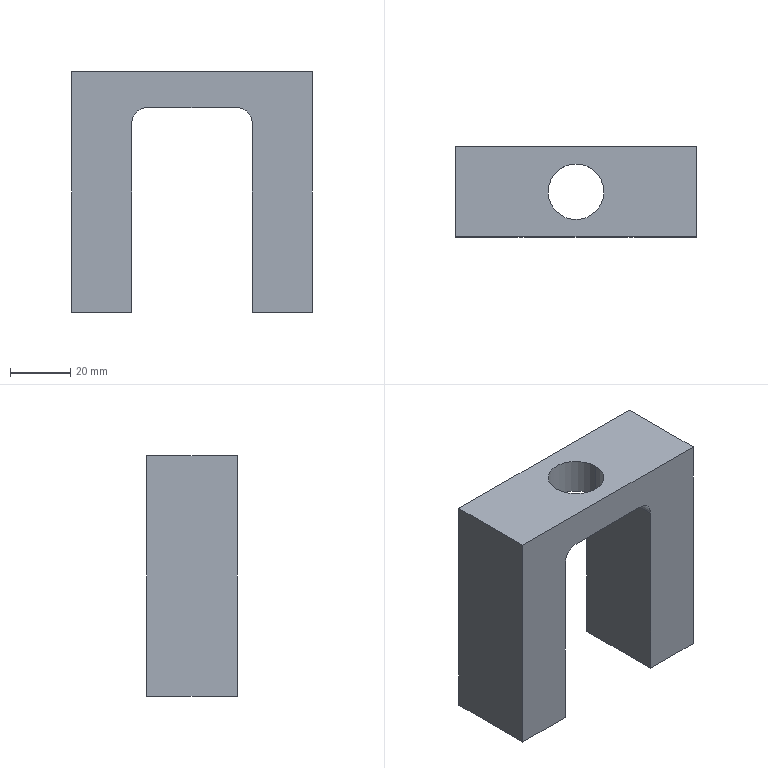Part | STEP file | 11-FG-SJ00311 | 1 solid | 22 faces | box 80 x 30 x 80 mm | volume 106888 mm3 | plane 10 | cylinder 8 | cone 4 | commonest cylinder face diameters 5 x4 10 x2 18.5 x2
STEP:
#1=CARTESIAN_POINT('',(-27.5,0.,15.));
#2=VERTEX_POINT('',#1);
#3=CARTESIAN_POINT('',(-32.5,0.,15.));
#4=VERTEX_POINT('',#3);
#5=CARTESIAN_POINT('',(-30.,0.,15.));
#6=DIRECTION('',(0.,0.,-1.));
#7=DIRECTION('',(-1.,0.,0.));
#8=AXIS2_PLACEMENT_3D('',#5,#6,#7);
#9=CIRCLE('',#8,2.5);
#10=EDGE_CURVE('',#2,#4,#9,.T.);
#11=ORIENTED_EDGE('',*,*,#10,.F.);
#12=CARTESIAN_POINT('',(-27.5,0.,0.));
#13=VERTEX_POINT('',#12);
#14=CARTESIAN_POINT('',(-27.5,0.,0.));
#15=DIRECTION('',(0.,0.,-1.));
#16=VECTOR('',#15,1000.);
#17=LINE('',#14,#16);
#18=EDGE_CURVE('',#2,#13,#17,.T.);
#19=ORIENTED_EDGE('',*,*,#18,.T.);
#20=CARTESIAN_POINT('',(-32.5,0.,0.));
#21=VERTEX_POINT('',#20);
#22=CARTESIAN_POINT('',(-30.,0.,0.));
#23=DIRECTION('',(0.,0.,-1.));
#24=DIRECTION('',(-1.,0.,0.));
#25=AXIS2_PLACEMENT_3D('',#22,#23,#24);
#26=CIRCLE('',#25,2.5);
#27=EDGE_CURVE('',#13,#21,#26,.T.);
#28=ORIENTED_EDGE('',*,*,#27,.T.);
#29=CARTESIAN_POINT('',(-32.5,0.,0.));
#30=DIRECTION('',(0.,0.,-1.));
#31=VECTOR('',#30,1000.);
#32=LINE('',#29,#31);
#33=EDGE_CURVE('',#4,#21,#32,.T.);
#34=ORIENTED_EDGE('',*,*,#33,.F.);
#35=EDGE_LOOP('',(#11,#19,#28,#34));
#36=FACE_OUTER_BOUND('',#35,.T.);
#37=CARTESIAN_POINT('',(-30.,0.,0.));
#38=DIRECTION('',(0.,0.,-1.));
#39=DIRECTION('',(-1.,0.,0.));
#40=AXIS2_PLACEMENT_3D('',#37,#38,#39);
#41=CYLINDRICAL_SURFACE('',#40,2.5);
#42=ADVANCED_FACE('',(#36),#41,.F.);
#43=CARTESIAN_POINT('',(-30.,0.,16.502));
#44=VERTEX_POINT('',#43);
#45=CARTESIAN_POINT('',(-32.5,0.,15.));
#46=DIRECTION('',(-0.8572,0.,-0.515));
#47=VECTOR('',#46,1000.);
#48=LINE('',#45,#47);
#49=EDGE_CURVE('',#44,#4,#48,.T.);
#50=ORIENTED_EDGE('',*,*,#49,.F.);
#51=CARTESIAN_POINT('',(-27.5,0.,15.));
#52=DIRECTION('',(0.8572,0.,-0.515));
#53=VECTOR('',#52,1000.);
#54=LINE('',#51,#53);
#55=EDGE_CURVE('',#44,#2,#54,.T.);
#56=ORIENTED_EDGE('',*,*,#55,.T.);
#57=ORIENTED_EDGE('',*,*,#10,.T.);
#58=EDGE_LOOP('',(#50,#56,#57));
#59=FACE_OUTER_BOUND('',#58,.T.);
#60=CARTESIAN_POINT('',(-30.,0.,15.));
#61=DIRECTION('',(0.,0.,-1.));
#62=DIRECTION('',(-1.,0.,0.));
#63=AXIS2_PLACEMENT_3D('',#60,#61,#62);
#64=CONICAL_SURFACE('',#63,2.5,1.03);
#65=ADVANCED_FACE('',(#59),#64,.F.);
#66=CARTESIAN_POINT('',(32.5,0.,15.));
#67=VERTEX_POINT('',#66);
#68=CARTESIAN_POINT('',(27.5,0.,15.));
#69=VERTEX_POINT('',#68);
#70=CARTESIAN_POINT('',(30.,0.,15.));
#71=DIRECTION('',(0.,0.,-1.));
#72=DIRECTION('',(-1.,0.,0.));
#73=AXIS2_PLACEMENT_3D('',#70,#71,#72);
#74=CIRCLE('',#73,2.5);
#75=EDGE_CURVE('',#67,#69,#74,.T.);
#76=ORIENTED_EDGE('',*,*,#75,.F.);
#77=CARTESIAN_POINT('',(32.5,0.,0.));
#78=VERTEX_POINT('',#77);
#79=CARTESIAN_POINT('',(32.5,0.,0.));
#80=DIRECTION('',(0.,0.,-1.));
#81=VECTOR('',#80,1000.);
#82=LINE('',#79,#81);
#83=EDGE_CURVE('',#67,#78,#82,.T.);
#84=ORIENTED_EDGE('',*,*,#83,.T.);
#85=CARTESIAN_POINT('',(27.5,0.,0.));
#86=VERTEX_POINT('',#85);
#87=CARTESIAN_POINT('',(30.,0.,0.));
#88=DIRECTION('',(0.,0.,-1.));
#89=DIRECTION('',(-1.,0.,0.));
#90=AXIS2_PLACEMENT_3D('',#87,#88,#89);
#91=CIRCLE('',#90,2.5);
#92=EDGE_CURVE('',#78,#86,#91,.T.);
#93=ORIENTED_EDGE('',*,*,#92,.T.);
#94=CARTESIAN_POINT('',(27.5,0.,0.));
#95=DIRECTION('',(0.,0.,-1.));
#96=VECTOR('',#95,1000.);
#97=LINE('',#94,#96);
#98=EDGE_CURVE('',#69,#86,#97,.T.);
#99=ORIENTED_EDGE('',*,*,#98,.F.);
#100=EDGE_LOOP('',(#76,#84,#93,#99));
#101=FACE_OUTER_BOUND('',#100,.T.);
#102=CARTESIAN_POINT('',(30.,0.,0.));
#103=DIRECTION('',(0.,0.,-1.));
#104=DIRECTION('',(-1.,0.,0.));
#105=AXIS2_PLACEMENT_3D('',#102,#103,#104);
#106=CYLINDRICAL_SURFACE('',#105,2.5);
#107=ADVANCED_FACE('',(#101),#106,.F.);
#108=CARTESIAN_POINT('',(30.,0.,16.502));
#109=VERTEX_POINT('',#108);
#110=CARTESIAN_POINT('',(27.5,0.,15.));
#111=DIRECTION('',(-0.8572,0.,-0.515));
#112=VECTOR('',#111,1000.);
#113=LINE('',#110,#112);
#114=EDGE_CURVE('',#109,#69,#113,.T.);
#115=ORIENTED_EDGE('',*,*,#114,.F.);
#116=CARTESIAN_POINT('',(32.5,0.,15.));
#117=DIRECTION('',(0.8572,0.,-0.515));
#118=VECTOR('',#117,1000.);
#119=LINE('',#116,#118);
#120=EDGE_CURVE('',#109,#67,#119,.T.);
#121=ORIENTED_EDGE('',*,*,#120,.T.);
#122=ORIENTED_EDGE('',*,*,#75,.T.);
#123=EDGE_LOOP('',(#115,#121,#122));
#124=FACE_OUTER_BOUND('',#123,.T.);
#125=CARTESIAN_POINT('',(30.,0.,15.));
#126=DIRECTION('',(0.,0.,-1.));
#127=DIRECTION('',(-1.,0.,0.));
#128=AXIS2_PLACEMENT_3D('',#125,#126,#127);
#129=CONICAL_SURFACE('',#128,2.5,1.03);
#130=ADVANCED_FACE('',(#124),#129,.F.);
#131=CARTESIAN_POINT('',(-9.25,0.,68.));
#132=VERTEX_POINT('',#131);
#133=CARTESIAN_POINT('',(9.25,0.,68.));
#134=VERTEX_POINT('',#133);
#135=CARTESIAN_POINT('',(0.,0.,68.));
#136=DIRECTION('',(0.,0.,1.));
#137=DIRECTION('',(1.,0.,0.));
#138=AXIS2_PLACEMENT_3D('',#135,#136,#137);
#139=CIRCLE('',#138,9.25);
#140=EDGE_CURVE('',#132,#134,#139,.T.);
#141=ORIENTED_EDGE('',*,*,#140,.F.);
#142=CARTESIAN_POINT('',(-9.25,0.,80.));
#143=VERTEX_POINT('',#142);
#144=CARTESIAN_POINT('',(-9.25,0.,80.));
#145=DIRECTION('',(0.,0.,1.));
#146=VECTOR('',#145,1000.);
#147=LINE('',#144,#146);
#148=EDGE_CURVE('',#132,#143,#147,.T.);
#149=ORIENTED_EDGE('',*,*,#148,.T.);
#150=CARTESIAN_POINT('',(9.25,0.,80.));
#151=VERTEX_POINT('',#150);
#152=CARTESIAN_POINT('',(0.,0.,80.));
#153=DIRECTION('',(0.,0.,1.));
#154=DIRECTION('',(1.,0.,0.));
#155=AXIS2_PLACEMENT_3D('',#152,#153,#154);
#156=CIRCLE('',#155,9.25);
#157=EDGE_CURVE('',#143,#151,#156,.T.);
#158=ORIENTED_EDGE('',*,*,#157,.T.);
#159=CARTESIAN_POINT('',(9.25,0.,80.));
#160=DIRECTION('',(0.,0.,1.));
#161=VECTOR('',#160,1000.);
#162=LINE('',#159,#161);
#163=EDGE_CURVE('',#134,#151,#162,.T.);
#164=ORIENTED_EDGE('',*,*,#163,.F.);
#165=EDGE_LOOP('',(#141,#149,#158,#164));
#166=FACE_OUTER_BOUND('',#165,.T.);
#167=CARTESIAN_POINT('',(0.,0.,80.));
#168=DIRECTION('',(0.,0.,1.));
#169=DIRECTION('',(1.,0.,0.));
#170=AXIS2_PLACEMENT_3D('',#167,#168,#169);
#171=CYLINDRICAL_SURFACE('',#170,9.25);
#172=ADVANCED_FACE('',(#166),#171,.F.);
#173=CARTESIAN_POINT('',(30.,0.,0.));
#174=DIRECTION('',(0.,0.,-1.));
#175=DIRECTION('',(-1.,0.,0.));
#176=AXIS2_PLACEMENT_3D('',#173,#174,#175);
#177=CIRCLE('',#176,2.5);
#178=EDGE_CURVE('',#86,#78,#177,.T.);
#179=ORIENTED_EDGE('',*,*,#178,.F.);
#180=ORIENTED_EDGE('',*,*,#92,.F.);
#181=EDGE_LOOP('',(#179,#180));
#182=FACE_BOUND('',#181,.T.);
#183=CARTESIAN_POINT('',(20.,-15.,0.));
#184=VERTEX_POINT('',#183);
#185=CARTESIAN_POINT('',(40.,-15.,0.));
#186=VERTEX_POINT('',#185);
#187=CARTESIAN_POINT('',(40.,-15.,0.));
#188=DIRECTION('',(1.,0.,0.));
#189=VECTOR('',#188,1000.);
#190=LINE('',#187,#189);
#191=EDGE_CURVE('',#184,#186,#190,.T.);
#192=ORIENTED_EDGE('',*,*,#191,.F.);
#193=CARTESIAN_POINT('',(20.,15.,0.));
#194=VERTEX_POINT('',#193);
#195=CARTESIAN_POINT('',(20.,0.,0.));
#196=DIRECTION('',(0.,1.,0.));
#197=VECTOR('',#196,1000.);
#198=LINE('',#195,#197);
#199=EDGE_CURVE('',#184,#194,#198,.T.);
#200=ORIENTED_EDGE('',*,*,#199,.T.);
#201=CARTESIAN_POINT('',(40.,15.,0.));
#202=VERTEX_POINT('',#201);
#203=CARTESIAN_POINT('',(40.,15.,0.));
#204=DIRECTION('',(-1.,0.,0.));
#205=VECTOR('',#204,1000.);
#206=LINE('',#203,#205);
#207=EDGE_CURVE('',#202,#194,#206,.T.);
#208=ORIENTED_EDGE('',*,*,#207,.F.);
#209=CARTESIAN_POINT('',(40.,-15.,0.));
#210=DIRECTION('',(0.,1.,0.));
#211=VECTOR('',#210,1000.);
#212=LINE('',#209,#211);
#213=EDGE_CURVE('',#186,#202,#212,.T.);
#214=ORIENTED_EDGE('',*,*,#213,.F.);
#215=EDGE_LOOP('',(#192,#200,#208,#214));
#216=FACE_OUTER_BOUND('',#215,.T.);
#217=CARTESIAN_POINT('',(0.,0.,0.));
#218=DIRECTION('',(0.,0.,1.));
#219=DIRECTION('',(1.,0.,0.));
#220=AXIS2_PLACEMENT_3D('',#217,#218,#219);
#221=PLANE('',#220);
#222=ADVANCED_FACE('',(#182,#216),#221,.F.);
#223=CARTESIAN_POINT('',(-40.,15.,0.));
#224=VERTEX_POINT('',#223);
#225=CARTESIAN_POINT('',(-40.,-15.,0.));
#226=VERTEX_POINT('',#225);
#227=CARTESIAN_POINT('',(-40.,-15.,0.));
#228=DIRECTION('',(0.,-1.,0.));
#229=VECTOR('',#228,1000.);
#230=LINE('',#227,#229);
#231=EDGE_CURVE('',#224,#226,#230,.T.);
#232=ORIENTED_EDGE('',*,*,#231,.T.);
#233=CARTESIAN_POINT('',(-40.,-15.,80.));
#234=VERTEX_POINT('',#233);
#235=CARTESIAN_POINT('',(-40.,-15.,80.));
#236=DIRECTION('',(0.,0.,-1.));
#237=VECTOR('',#236,1000.);
#238=LINE('',#235,#237);
#239=EDGE_CURVE('',#234,#226,#238,.T.);
#240=ORIENTED_EDGE('',*,*,#239,.F.);
#241=CARTESIAN_POINT('',(-40.,15.,80.));
#242=VERTEX_POINT('',#241);
#243=CARTESIAN_POINT('',(-40.,-15.,80.));
#244=DIRECTION('',(0.,-1.,0.));
#245=VECTOR('',#244,1000.);
#246=LINE('',#243,#245);
#247=EDGE_CURVE('',#242,#234,#246,.T.);
#248=ORIENTED_EDGE('',*,*,#247,.F.);
#249=CARTESIAN_POINT('',(-40.,15.,80.));
#250=DIRECTION('',(0.,0.,-1.));
#251=VECTOR('',#250,1000.);
#252=LINE('',#249,#251);
#253=EDGE_CURVE('',#242,#224,#252,.T.);
#254=ORIENTED_EDGE('',*,*,#253,.T.);
#255=EDGE_LOOP('',(#232,#240,#248,#254));
#256=FACE_OUTER_BOUND('',#255,.T.);
#257=CARTESIAN_POINT('',(-40.,-15.,80.));
#258=DIRECTION('',(1.,0.,0.));
#259=DIRECTION('',(0.,0.,-1.));
#260=AXIS2_PLACEMENT_3D('',#257,#258,#259);
#261=PLANE('',#260);
#262=ADVANCED_FACE('',(#256),#261,.F.);
#263=CARTESIAN_POINT('',(20.,-15.,63.));
#264=VERTEX_POINT('',#263);
#265=CARTESIAN_POINT('',(15.,-15.,68.));
#266=VERTEX_POINT('',#265);
#267=CARTESIAN_POINT('',(15.,-15.,63.));
#268=DIRECTION('',(0.,-1.,0.));
#269=DIRECTION('',(1.,0.,0.));
#270=AXIS2_PLACEMENT_3D('',#267,#268,#269);
#271=CIRCLE('',#270,5.);
#272=EDGE_CURVE('',#264,#266,#271,.T.);
#273=ORIENTED_EDGE('',*,*,#272,.F.);
#274=CARTESIAN_POINT('',(20.,-15.,-68.));
#275=DIRECTION('',(0.,0.,1.));
#276=VECTOR('',#275,1000.);
#277=LINE('',#274,#276);
#278=EDGE_CURVE('',#184,#264,#277,.T.);
#279=ORIENTED_EDGE('',*,*,#278,.F.);
#280=ORIENTED_EDGE('',*,*,#191,.T.);
#281=CARTESIAN_POINT('',(40.,-15.,80.));
#282=VERTEX_POINT('',#281);
#283=CARTESIAN_POINT('',(40.,-15.,80.));
#284=DIRECTION('',(0.,0.,-1.));
#285=VECTOR('',#284,1000.);
#286=LINE('',#283,#285);
#287=EDGE_CURVE('',#282,#186,#286,.T.);
#288=ORIENTED_EDGE('',*,*,#287,.F.);
#289=CARTESIAN_POINT('',(40.,-15.,80.));
#290=DIRECTION('',(1.,0.,0.));
#291=VECTOR('',#290,1000.);
#292=LINE('',#289,#291);
#293=EDGE_CURVE('',#234,#282,#292,.T.);
#294=ORIENTED_EDGE('',*,*,#293,.F.);
#295=ORIENTED_EDGE('',*,*,#239,.T.);
#296=CARTESIAN_POINT('',(-20.,-15.,0.));
#297=VERTEX_POINT('',#296);
#298=CARTESIAN_POINT('',(40.,-15.,0.));
#299=DIRECTION('',(1.,0.,0.));
#300=VECTOR('',#299,1000.);
#301=LINE('',#298,#300);
#302=EDGE_CURVE('',#226,#297,#301,.T.);
#303=ORIENTED_EDGE('',*,*,#302,.T.);
#304=CARTESIAN_POINT('',(-20.,-15.,63.));
#305=VERTEX_POINT('',#304);
#306=CARTESIAN_POINT('',(-20.,-15.,-68.));
#307=DIRECTION('',(0.,0.,-1.));
#308=VECTOR('',#307,1000.);
#309=LINE('',#306,#308);
#310=EDGE_CURVE('',#305,#297,#309,.T.);
#311=ORIENTED_EDGE('',*,*,#310,.F.);
#312=CARTESIAN_POINT('',(-15.,-15.,68.));
#313=VERTEX_POINT('',#312);
#314=CARTESIAN_POINT('',(-15.,-15.,63.));
#315=DIRECTION('',(0.,-1.,0.));
#316=DIRECTION('',(1.,0.,0.));
#317=AXIS2_PLACEMENT_3D('',#314,#315,#316);
#318=CIRCLE('',#317,5.);
#319=EDGE_CURVE('',#313,#305,#318,.T.);
#320=ORIENTED_EDGE('',*,*,#319,.F.);
#321=CARTESIAN_POINT('',(15.,-15.,68.));
#322=DIRECTION('',(-1.,0.,0.));
#323=VECTOR('',#322,1000.);
#324=LINE('',#321,#323);
#325=EDGE_CURVE('',#266,#313,#324,.T.);
#326=ORIENTED_EDGE('',*,*,#325,.F.);
#327=EDGE_LOOP('',(#273,#279,#280,#288,#294,#295,#303,#311,#320,#326));
#328=FACE_OUTER_BOUND('',#327,.T.);
#329=CARTESIAN_POINT('',(40.,-15.,80.));
#330=DIRECTION('',(0.,1.,0.));
#331=DIRECTION('',(-1.,0.,0.));
#332=AXIS2_PLACEMENT_3D('',#329,#330,#331);
#333=PLANE('',#332);
#334=ADVANCED_FACE('',(#328),#333,.F.);
#335=ORIENTED_EDGE('',*,*,#213,.T.);
#336=CARTESIAN_POINT('',(40.,15.,80.));
#337=VERTEX_POINT('',#336);
#338=CARTESIAN_POINT('',(40.,15.,80.));
#339=DIRECTION('',(0.,0.,-1.));
#340=VECTOR('',#339,1000.);
#341=LINE('',#338,#340);
#342=EDGE_CURVE('',#337,#202,#341,.T.);
#343=ORIENTED_EDGE('',*,*,#342,.F.);
#344=CARTESIAN_POINT('',(40.,-15.,80.));
#345=DIRECTION('',(0.,1.,0.));
#346=VECTOR('',#345,1000.);
#347=LINE('',#344,#346);
#348=EDGE_CURVE('',#282,#337,#347,.T.);
#349=ORIENTED_EDGE('',*,*,#348,.F.);
#350=ORIENTED_EDGE('',*,*,#287,.T.);
#351=EDGE_LOOP('',(#335,#343,#349,#350));
#352=FACE_OUTER_BOUND('',#351,.T.);
#353=CARTESIAN_POINT('',(40.,-15.,80.));
#354=DIRECTION('',(-1.,0.,0.));
#355=DIRECTION('',(0.,0.,1.));
#356=AXIS2_PLACEMENT_3D('',#353,#354,#355);
#357=PLANE('',#356);
#358=ADVANCED_FACE('',(#352),#357,.F.);
#359=ORIENTED_EDGE('',*,*,#207,.T.);
#360=CARTESIAN_POINT('',(20.,15.,63.));
#361=VERTEX_POINT('',#360);
#362=CARTESIAN_POINT('',(20.,15.,-68.));
#363=DIRECTION('',(0.,0.,1.));
#364=VECTOR('',#363,1000.);
#365=LINE('',#362,#364);
#366=EDGE_CURVE('',#194,#361,#365,.T.);
#367=ORIENTED_EDGE('',*,*,#366,.T.);
#368=CARTESIAN_POINT('',(15.,15.,68.));
#369=VERTEX_POINT('',#368);
#370=CARTESIAN_POINT('',(15.,15.,63.));
#371=DIRECTION('',(0.,-1.,0.));
#372=DIRECTION('',(1.,0.,0.));
#373=AXIS2_PLACEMENT_3D('',#370,#371,#372);
#374=CIRCLE('',#373,5.);
#375=EDGE_CURVE('',#361,#369,#374,.T.);
#376=ORIENTED_EDGE('',*,*,#375,.T.);
#377=CARTESIAN_POINT('',(-15.,15.,68.));
#378=VERTEX_POINT('',#377);
#379=CARTESIAN_POINT('',(15.,15.,68.));
#380=DIRECTION('',(-1.,0.,0.));
#381=VECTOR('',#380,1000.);
#382=LINE('',#379,#381);
#383=EDGE_CURVE('',#369,#378,#382,.T.);
#384=ORIENTED_EDGE('',*,*,#383,.T.);
#385=CARTESIAN_POINT('',(-20.,15.,63.));
#386=VERTEX_POINT('',#385);
#387=CARTESIAN_POINT('',(-15.,15.,63.));
#388=DIRECTION('',(0.,-1.,0.));
#389=DIRECTION('',(1.,0.,0.));
#390=AXIS2_PLACEMENT_3D('',#387,#388,#389);
#391=CIRCLE('',#390,5.);
#392=EDGE_CURVE('',#378,#386,#391,.T.);
#393=ORIENTED_EDGE('',*,*,#392,.T.);
#394=CARTESIAN_POINT('',(-20.,15.,0.));
#395=VERTEX_POINT('',#394);
#396=CARTESIAN_POINT('',(-20.,15.,-68.));
#397=DIRECTION('',(0.,0.,-1.));
#398=VECTOR('',#397,1000.);
#399=LINE('',#396,#398);
#400=EDGE_CURVE('',#386,#395,#399,.T.);
#401=ORIENTED_EDGE('',*,*,#400,.T.);
#402=CARTESIAN_POINT('',(40.,15.,0.));
#403=DIRECTION('',(-1.,0.,0.));
#404=VECTOR('',#403,1000.);
#405=LINE('',#402,#404);
#406=EDGE_CURVE('',#395,#224,#405,.T.);
#407=ORIENTED_EDGE('',*,*,#406,.T.);
#408=ORIENTED_EDGE('',*,*,#253,.F.);
#409=CARTESIAN_POINT('',(40.,15.,80.));
#410=DIRECTION('',(-1.,0.,0.));
#411=VECTOR('',#410,1000.);
#412=LINE('',#409,#411);
#413=EDGE_CURVE('',#337,#242,#412,.T.);
#414=ORIENTED_EDGE('',*,*,#413,.F.);
#415=ORIENTED_EDGE('',*,*,#342,.T.);
#416=EDGE_LOOP('',(#359,#367,#376,#384,#393,#401,#407,#408,#414,#415));
#417=FACE_OUTER_BOUND('',#416,.T.);
#418=CARTESIAN_POINT('',(40.,15.,80.));
#419=DIRECTION('',(0.,-1.,0.));
#420=DIRECTION('',(1.,0.,0.));
#421=AXIS2_PLACEMENT_3D('',#418,#419,#420);
#422=PLANE('',#421);
#423=ADVANCED_FACE('',(#417),#422,.F.);
#424=CARTESIAN_POINT('',(0.,0.,80.));
#425=DIRECTION('',(0.,0.,1.));
#426=DIRECTION('',(1.,0.,0.));
#427=AXIS2_PLACEMENT_3D('',#424,#425,#426);
#428=CIRCLE('',#427,9.25);
#429=EDGE_CURVE('',#151,#143,#428,.T.);
#430=ORIENTED_EDGE('',*,*,#429,.F.);
#431=ORIENTED_EDGE('',*,*,#157,.F.);
#432=EDGE_LOOP('',(#430,#431));
#433=FACE_BOUND('',#432,.T.);
#434=ORIENTED_EDGE('',*,*,#247,.T.);
#435=ORIENTED_EDGE('',*,*,#293,.T.);
#436=ORIENTED_EDGE('',*,*,#348,.T.);
#437=ORIENTED_EDGE('',*,*,#413,.T.);
#438=EDGE_LOOP('',(#434,#435,#436,#437));
#439=FACE_OUTER_BOUND('',#438,.T.);
#440=CARTESIAN_POINT('',(0.,0.,80.));
#441=DIRECTION('',(0.,0.,1.));
#442=DIRECTION('',(1.,0.,0.));
#443=AXIS2_PLACEMENT_3D('',#440,#441,#442);
#444=PLANE('',#443);
#445=ADVANCED_FACE('',(#433,#439),#444,.T.);
#446=CARTESIAN_POINT('',(-30.,0.,0.));
#447=DIRECTION('',(0.,0.,-1.));
#448=DIRECTION('',(-1.,0.,0.));
#449=AXIS2_PLACEMENT_3D('',#446,#447,#448);
#450=CIRCLE('',#449,2.5);
#451=EDGE_CURVE('',#21,#13,#450,.T.);
#452=ORIENTED_EDGE('',*,*,#451,.F.);
#453=ORIENTED_EDGE('',*,*,#27,.F.);
#454=EDGE_LOOP('',(#452,#453));
#455=FACE_BOUND('',#454,.T.);
#456=ORIENTED_EDGE('',*,*,#406,.F.);
#457=CARTESIAN_POINT('',(-20.,0.,0.));
#458=DIRECTION('',(0.,-1.,0.));
#459=VECTOR('',#458,1000.);
#460=LINE('',#457,#459);
#461=EDGE_CURVE('',#395,#297,#460,.T.);
#462=ORIENTED_EDGE('',*,*,#461,.T.);
#463=ORIENTED_EDGE('',*,*,#302,.F.);
#464=ORIENTED_EDGE('',*,*,#231,.F.);
#465=EDGE_LOOP('',(#456,#462,#463,#464));
#466=FACE_OUTER_BOUND('',#465,.T.);
#467=CARTESIAN_POINT('',(0.,0.,0.));
#468=DIRECTION('',(0.,0.,1.));
#469=DIRECTION('',(1.,0.,0.));
#470=AXIS2_PLACEMENT_3D('',#467,#468,#469);
#471=PLANE('',#470);
#472=ADVANCED_FACE('',(#455,#466),#471,.F.);
#473=ORIENTED_EDGE('',*,*,#278,.T.);
#474=CARTESIAN_POINT('',(20.,15.,63.));
#475=DIRECTION('',(0.,-1.,0.));
#476=VECTOR('',#475,1000.);
#477=LINE('',#474,#476);
#478=EDGE_CURVE('',#361,#264,#477,.T.);
#479=ORIENTED_EDGE('',*,*,#478,.F.);
#480=ORIENTED_EDGE('',*,*,#366,.F.);
#481=ORIENTED_EDGE('',*,*,#199,.F.);
#482=EDGE_LOOP('',(#473,#479,#480,#481));
#483=FACE_OUTER_BOUND('',#482,.T.);
#484=CARTESIAN_POINT('',(20.,15.,-68.));
#485=DIRECTION('',(1.,0.,0.));
#486=DIRECTION('',(0.,1.,0.));
#487=AXIS2_PLACEMENT_3D('',#484,#485,#486);
#488=PLANE('',#487);
#489=ADVANCED_FACE('',(#483),#488,.F.);
#490=ORIENTED_EDGE('',*,*,#400,.F.);
#491=CARTESIAN_POINT('',(-20.,15.,63.));
#492=DIRECTION('',(0.,-1.,0.));
#493=VECTOR('',#492,1000.);
#494=LINE('',#491,#493);
#495=EDGE_CURVE('',#386,#305,#494,.T.);
#496=ORIENTED_EDGE('',*,*,#495,.T.);
#497=ORIENTED_EDGE('',*,*,#310,.T.);
#498=ORIENTED_EDGE('',*,*,#461,.F.);
#499=EDGE_LOOP('',(#490,#496,#497,#498));
#500=FACE_OUTER_BOUND('',#499,.T.);
#501=CARTESIAN_POINT('',(-20.,15.,-68.));
#502=DIRECTION('',(-1.,0.,0.));
#503=DIRECTION('',(0.,-1.,0.));
#504=AXIS2_PLACEMENT_3D('',#501,#502,#503);
#505=PLANE('',#504);
#506=ADVANCED_FACE('',(#500),#505,.F.);
#507=ORIENTED_EDGE('',*,*,#319,.T.);
#508=ORIENTED_EDGE('',*,*,#495,.F.);
#509=ORIENTED_EDGE('',*,*,#392,.F.);
#510=CARTESIAN_POINT('',(-15.,15.,68.));
#511=DIRECTION('',(0.,-1.,0.));
#512=VECTOR('',#511,1000.);
#513=LINE('',#510,#512);
#514=EDGE_CURVE('',#378,#313,#513,.T.);
#515=ORIENTED_EDGE('',*,*,#514,.T.);
#516=EDGE_LOOP('',(#507,#508,#509,#515));
#517=FACE_OUTER_BOUND('',#516,.T.);
#518=CARTESIAN_POINT('',(-15.,15.,63.));
#519=DIRECTION('',(0.,-1.,0.));
#520=DIRECTION('',(1.,0.,0.));
#521=AXIS2_PLACEMENT_3D('',#518,#519,#520);
#522=CYLINDRICAL_SURFACE('',#521,5.);
#523=ADVANCED_FACE('',(#517),#522,.F.);
#524=CARTESIAN_POINT('',(0.,0.,68.));
#525=DIRECTION('',(0.,0.,1.));
#526=DIRECTION('',(1.,0.,0.));
#527=AXIS2_PLACEMENT_3D('',#524,#525,#526);
#528=CIRCLE('',#527,9.25);
#529=EDGE_CURVE('',#134,#132,#528,.T.);
#530=ORIENTED_EDGE('',*,*,#529,.T.);
#531=ORIENTED_EDGE('',*,*,#140,.T.);
#532=EDGE_LOOP('',(#530,#531));
#533=FACE_BOUND('',#532,.T.);
#534=ORIENTED_EDGE('',*,*,#325,.T.);
#535=ORIENTED_EDGE('',*,*,#514,.F.);
#536=ORIENTED_EDGE('',*,*,#383,.F.);
#537=CARTESIAN_POINT('',(15.,15.,68.));
#538=DIRECTION('',(0.,-1.,0.));
#539=VECTOR('',#538,1000.);
#540=LINE('',#537,#539);
#541=EDGE_CURVE('',#369,#266,#540,.T.);
#542=ORIENTED_EDGE('',*,*,#541,.T.);
#543=EDGE_LOOP('',(#534,#535,#536,#542));
#544=FACE_OUTER_BOUND('',#543,.T.);
#545=CARTESIAN_POINT('',(15.,15.,68.));
#546=DIRECTION('',(0.,0.,1.));
#547=DIRECTION('',(1.,0.,0.));
#548=AXIS2_PLACEMENT_3D('',#545,#546,#547);
#549=PLANE('',#548);
#550=ADVANCED_FACE('',(#533,#544),#549,.F.);
#551=ORIENTED_EDGE('',*,*,#272,.T.);
#552=ORIENTED_EDGE('',*,*,#541,.F.);
#553=ORIENTED_EDGE('',*,*,#375,.F.);
#554=ORIENTED_EDGE('',*,*,#478,.T.);
#555=EDGE_LOOP('',(#551,#552,#553,#554));
#556=FACE_OUTER_BOUND('',#555,.T.);
#557=CARTESIAN_POINT('',(15.,15.,63.));
#558=DIRECTION('',(0.,-1.,0.));
#559=DIRECTION('',(1.,0.,0.));
#560=AXIS2_PLACEMENT_3D('',#557,#558,#559);
#561=CYLINDRICAL_SURFACE('',#560,5.);
#562=ADVANCED_FACE('',(#556),#561,.F.);
#563=ORIENTED_EDGE('',*,*,#148,.F.);
#564=ORIENTED_EDGE('',*,*,#529,.F.);
#565=ORIENTED_EDGE('',*,*,#163,.T.);
#566=ORIENTED_EDGE('',*,*,#429,.T.);
#567=EDGE_LOOP('',(#563,#564,#565,#566));
#568=FACE_OUTER_BOUND('',#567,.T.);
#569=CARTESIAN_POINT('',(0.,0.,80.));
#570=DIRECTION('',(0.,0.,1.));
#571=DIRECTION('',(1.,0.,0.));
#572=AXIS2_PLACEMENT_3D('',#569,#570,#571);
#573=CYLINDRICAL_SURFACE('',#572,9.25);
#574=ADVANCED_FACE('',(#568),#573,.F.);
#575=ORIENTED_EDGE('',*,*,#120,.F.);
#576=ORIENTED_EDGE('',*,*,#114,.T.);
#577=CARTESIAN_POINT('',(30.,0.,15.));
#578=DIRECTION('',(0.,0.,-1.));
#579=DIRECTION('',(-1.,0.,0.));
#580=AXIS2_PLACEMENT_3D('',#577,#578,#579);
#581=CIRCLE('',#580,2.5);
#582=EDGE_CURVE('',#69,#67,#581,.T.);
#583=ORIENTED_EDGE('',*,*,#582,.T.);
#584=EDGE_LOOP('',(#575,#576,#583));
#585=FACE_OUTER_BOUND('',#584,.T.);
#586=CARTESIAN_POINT('',(30.,0.,15.));
#587=DIRECTION('',(0.,0.,-1.));
#588=DIRECTION('',(-1.,0.,0.));
#589=AXIS2_PLACEMENT_3D('',#586,#587,#588);
#590=CONICAL_SURFACE('',#589,2.5,1.03);
#591=ADVANCED_FACE('',(#585),#590,.F.);
#592=ORIENTED_EDGE('',*,*,#83,.F.);
#593=ORIENTED_EDGE('',*,*,#582,.F.);
#594=ORIENTED_EDGE('',*,*,#98,.T.);
#595=ORIENTED_EDGE('',*,*,#178,.T.);
#596=EDGE_LOOP('',(#592,#593,#594,#595));
#597=FACE_OUTER_BOUND('',#596,.T.);
#598=CARTESIAN_POINT('',(30.,0.,0.));
#599=DIRECTION('',(0.,0.,-1.));
#600=DIRECTION('',(-1.,0.,0.));
#601=AXIS2_PLACEMENT_3D('',#598,#599,#600);
#602=CYLINDRICAL_SURFACE('',#601,2.5);
#603=ADVANCED_FACE('',(#597),#602,.F.);
#604=ORIENTED_EDGE('',*,*,#55,.F.);
#605=ORIENTED_EDGE('',*,*,#49,.T.);
#606=CARTESIAN_POINT('',(-30.,0.,15.));
#607=DIRECTION('',(0.,0.,-1.));
#608=DIRECTION('',(-1.,0.,0.));
#609=AXIS2_PLACEMENT_3D('',#606,#607,#608);
#610=CIRCLE('',#609,2.5);
#611=EDGE_CURVE('',#4,#2,#610,.T.);
#612=ORIENTED_EDGE('',*,*,#611,.T.);
#613=EDGE_LOOP('',(#604,#605,#612));
#614=FACE_OUTER_BOUND('',#613,.T.);
#615=CARTESIAN_POINT('',(-30.,0.,15.));
#616=DIRECTION('',(0.,0.,-1.));
#617=DIRECTION('',(-1.,0.,0.));
#618=AXIS2_PLACEMENT_3D('',#615,#616,#617);
#619=CONICAL_SURFACE('',#618,2.5,1.03);
#620=ADVANCED_FACE('',(#614),#619,.F.);
#621=ORIENTED_EDGE('',*,*,#18,.F.);
#622=ORIENTED_EDGE('',*,*,#611,.F.);
#623=ORIENTED_EDGE('',*,*,#33,.T.);
#624=ORIENTED_EDGE('',*,*,#451,.T.);
#625=EDGE_LOOP('',(#621,#622,#623,#624));
#626=FACE_OUTER_BOUND('',#625,.T.);
#627=CARTESIAN_POINT('',(-30.,0.,0.));
#628=DIRECTION('',(0.,0.,-1.));
#629=DIRECTION('',(-1.,0.,0.));
#630=AXIS2_PLACEMENT_3D('',#627,#628,#629);
#631=CYLINDRICAL_SURFACE('',#630,2.5);
#632=ADVANCED_FACE('',(#626),#631,.F.);
#633=CLOSED_SHELL('',(#42,#65,#107,#130,#172,#222,#262,#334,#358,#423,#445,#472,#489,#506,#523,#550,#562,#574,#591,#603,#620,#632));
#634=MANIFOLD_SOLID_BREP('',#633);
#635=CARTESIAN_POINT('',(0.,0.,0.));
#636=DIRECTION('',(0.,0.,1.));
#637=DIRECTION('',(1.,0.,0.));
#638=AXIS2_PLACEMENT_3D('',#635,#636,#637);
#639=(LENGTH_UNIT()NAMED_UNIT(*)SI_UNIT(.MILLI.,.METRE.));
#640=UNCERTAINTY_MEASURE_WITH_UNIT(LENGTH_MEASURE(0.00001),#639,'','');
#641=(NAMED_UNIT(*)PLANE_ANGLE_UNIT()SI_UNIT($,.RADIAN.));
#642=(NAMED_UNIT(*)SI_UNIT($,.STERADIAN.)SOLID_ANGLE_UNIT());
#643=(GEOMETRIC_REPRESENTATION_CONTEXT(3)GLOBAL_UNCERTAINTY_ASSIGNED_CONTEXT((#640))GLOBAL_UNIT_ASSIGNED_CONTEXT((#639,#641,#642))REPRESENTATION_CONTEXT('',''));
#644=ADVANCED_BREP_SHAPE_REPRESENTATION('',(#634,#638),#643);